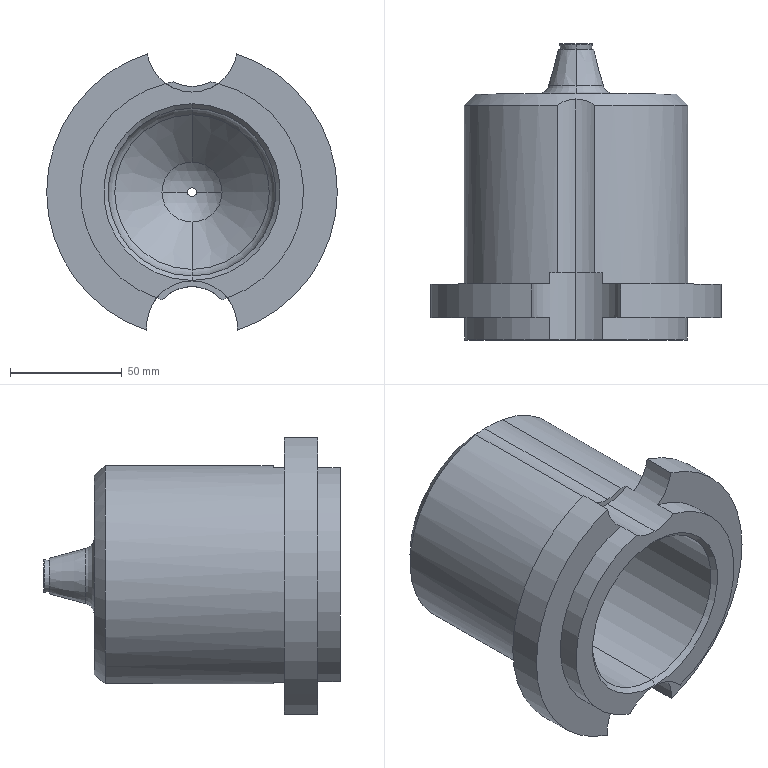Part | STEP file | 1 solid | 44 faces | box 130 x 132.5 x 123.637 mm | volume 522073 mm3 | cylinder 14 | cone 13 | plane 9 | torus 6 | sphere 2 | commonest cylinder face diameters 35.5 x3 40.5 x3 75 x2 99.8 x2 100 x2 130 x2